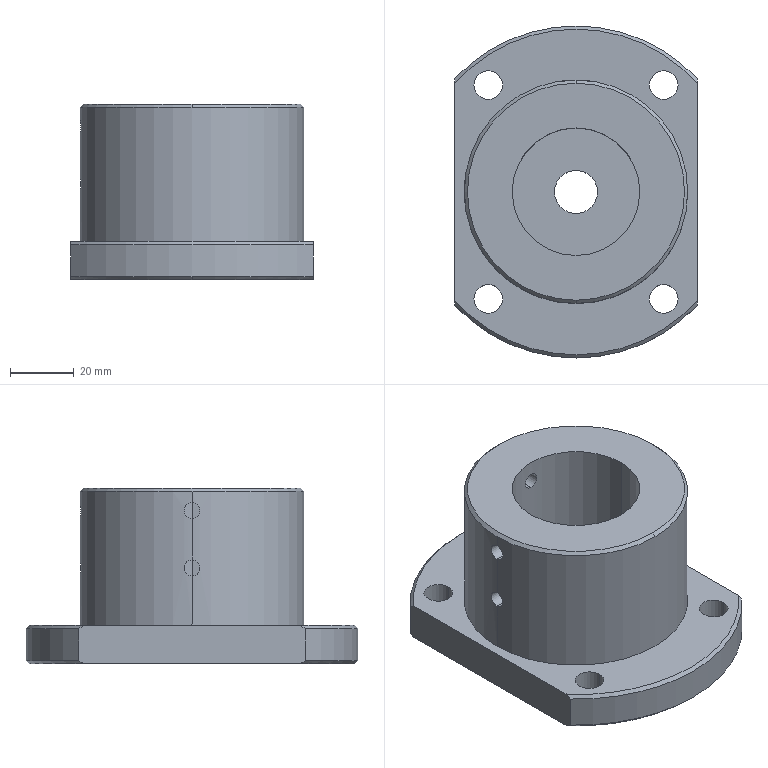Part | STEP file | fBY02F02M-00-01A | 1 solid | 40 faces | box 76 x 104 x 55 mm | volume 203193 mm3 | cylinder 26 | cone 7 | plane 7 | commonest cylinder face diameters 5 x8 9 x8 13.5 x2 20 x2 40 x2 70 x2